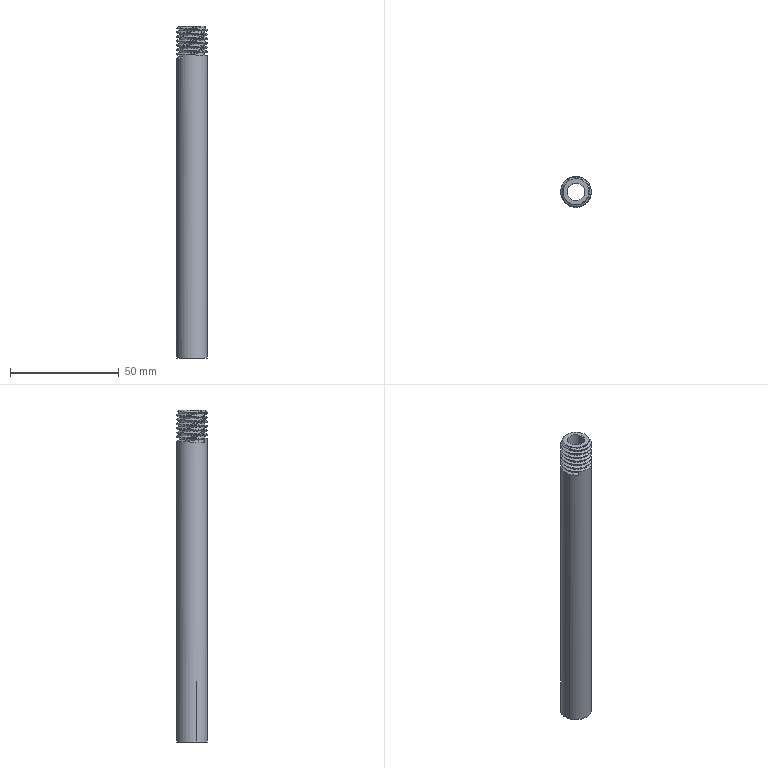Part | SolidWorks | features BaseBody 1 | 1 solid | 41 faces | box 14 x 14 x 152.5 mm | volume 15477 mm3 | cylinder 33 | cone 3 | plane 3 | spline 2 | commonest cylinder face diameters 12 x16 14 x15 8 x2